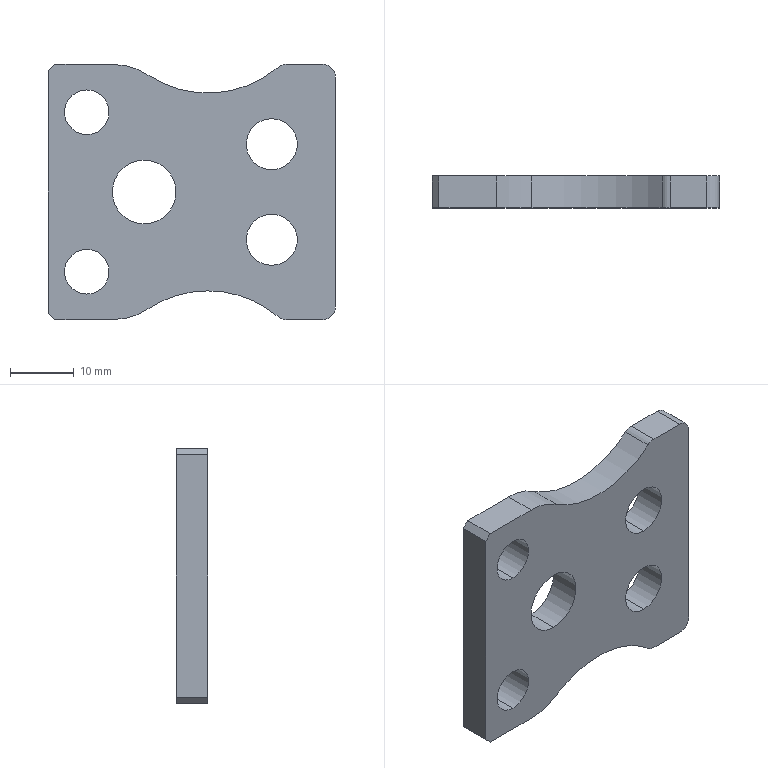Part | SolidWorks | features BaseBody 1 | 1 solid | 29 faces | box 45 x 5 x 40 mm | volume 6983 mm3 | cylinder 19 | plane 10 | commonest cylinder face diameters 4 x4 7 x4 8 x4 34 x3 10 x2 20 x2
STEP:
#1=CARTESIAN_POINT('',(147.5,25.,-3.5));
#2=VERTEX_POINT('',#1);
#3=CARTESIAN_POINT('',(147.5,25.,-11.5));
#4=VERTEX_POINT('',#3);
#5=CARTESIAN_POINT('',(147.5,25.,-7.5));
#6=DIRECTION('',(0.,-1.,0.));
#7=DIRECTION('',(0.,0.,-1.));
#8=AXIS2_PLACEMENT_3D('',#5,#6,#7);
#9=CIRCLE('',#8,4.);
#10=EDGE_CURVE('',#2,#4,#9,.T.);
#11=ORIENTED_EDGE('',*,*,#10,.T.);
#12=CARTESIAN_POINT('',(147.5,30.,-11.5));
#13=VERTEX_POINT('',#12);
#14=CARTESIAN_POINT('',(147.5,25.,-11.5));
#15=DIRECTION('',(0.,1.,0.));
#16=VECTOR('',#15,1000.);
#17=LINE('',#14,#16);
#18=EDGE_CURVE('',#4,#13,#17,.T.);
#19=ORIENTED_EDGE('',*,*,#18,.T.);
#20=CARTESIAN_POINT('',(147.5,30.,-3.5));
#21=VERTEX_POINT('',#20);
#22=CARTESIAN_POINT('',(147.5,30.,-7.5));
#23=DIRECTION('',(0.,-1.,0.));
#24=DIRECTION('',(0.,0.,-1.));
#25=AXIS2_PLACEMENT_3D('',#22,#23,#24);
#26=CIRCLE('',#25,4.);
#27=EDGE_CURVE('',#21,#13,#26,.T.);
#28=ORIENTED_EDGE('',*,*,#27,.F.);
#29=CARTESIAN_POINT('',(147.5,25.,-3.5));
#30=DIRECTION('',(0.,1.,0.));
#31=VECTOR('',#30,1000.);
#32=LINE('',#29,#31);
#33=EDGE_CURVE('',#2,#21,#32,.T.);
#34=ORIENTED_EDGE('',*,*,#33,.F.);
#35=EDGE_LOOP('',(#11,#19,#28,#34));
#36=FACE_OUTER_BOUND('',#35,.T.);
#37=CARTESIAN_POINT('',(147.5,25.,-7.5));
#38=DIRECTION('',(0.,1.,0.));
#39=DIRECTION('',(0.,0.,1.));
#40=AXIS2_PLACEMENT_3D('',#37,#38,#39);
#41=CYLINDRICAL_SURFACE('',#40,4.);
#42=ADVANCED_FACE('',(#36),#41,.F.);
#43=CARTESIAN_POINT('',(147.5,25.,11.5));
#44=VERTEX_POINT('',#43);
#45=CARTESIAN_POINT('',(147.5,25.,3.5));
#46=VERTEX_POINT('',#45);
#47=CARTESIAN_POINT('',(147.5,25.,7.5));
#48=DIRECTION('',(0.,-1.,0.));
#49=DIRECTION('',(0.,0.,-1.));
#50=AXIS2_PLACEMENT_3D('',#47,#48,#49);
#51=CIRCLE('',#50,4.);
#52=EDGE_CURVE('',#44,#46,#51,.T.);
#53=ORIENTED_EDGE('',*,*,#52,.T.);
#54=CARTESIAN_POINT('',(147.5,30.,3.5));
#55=VERTEX_POINT('',#54);
#56=CARTESIAN_POINT('',(147.5,25.,3.5));
#57=DIRECTION('',(0.,1.,0.));
#58=VECTOR('',#57,1000.);
#59=LINE('',#56,#58);
#60=EDGE_CURVE('',#46,#55,#59,.T.);
#61=ORIENTED_EDGE('',*,*,#60,.T.);
#62=CARTESIAN_POINT('',(147.5,30.,11.5));
#63=VERTEX_POINT('',#62);
#64=CARTESIAN_POINT('',(147.5,30.,7.5));
#65=DIRECTION('',(0.,-1.,0.));
#66=DIRECTION('',(0.,0.,-1.));
#67=AXIS2_PLACEMENT_3D('',#64,#65,#66);
#68=CIRCLE('',#67,4.);
#69=EDGE_CURVE('',#63,#55,#68,.T.);
#70=ORIENTED_EDGE('',*,*,#69,.F.);
#71=CARTESIAN_POINT('',(147.5,25.,11.5));
#72=DIRECTION('',(0.,1.,0.));
#73=VECTOR('',#72,1000.);
#74=LINE('',#71,#73);
#75=EDGE_CURVE('',#44,#63,#74,.T.);
#76=ORIENTED_EDGE('',*,*,#75,.F.);
#77=EDGE_LOOP('',(#53,#61,#70,#76));
#78=FACE_OUTER_BOUND('',#77,.T.);
#79=CARTESIAN_POINT('',(147.5,25.,7.5));
#80=DIRECTION('',(0.,1.,0.));
#81=DIRECTION('',(0.,0.,1.));
#82=AXIS2_PLACEMENT_3D('',#79,#80,#81);
#83=CYLINDRICAL_SURFACE('',#82,4.);
#84=ADVANCED_FACE('',(#78),#83,.F.);
#85=CARTESIAN_POINT('',(127.5,25.,5.));
#86=VERTEX_POINT('',#85);
#87=CARTESIAN_POINT('',(127.5,25.,-5.));
#88=VERTEX_POINT('',#87);
#89=CARTESIAN_POINT('',(127.5,25.,0.));
#90=DIRECTION('',(0.,-1.,0.));
#91=DIRECTION('',(0.,0.,-1.));
#92=AXIS2_PLACEMENT_3D('',#89,#90,#91);
#93=CIRCLE('',#92,5.);
#94=EDGE_CURVE('',#86,#88,#93,.T.);
#95=ORIENTED_EDGE('',*,*,#94,.T.);
#96=CARTESIAN_POINT('',(127.5,30.,-5.));
#97=VERTEX_POINT('',#96);
#98=CARTESIAN_POINT('',(127.5,25.,-5.));
#99=DIRECTION('',(0.,1.,0.));
#100=VECTOR('',#99,1000.);
#101=LINE('',#98,#100);
#102=EDGE_CURVE('',#88,#97,#101,.T.);
#103=ORIENTED_EDGE('',*,*,#102,.T.);
#104=CARTESIAN_POINT('',(127.5,30.,5.));
#105=VERTEX_POINT('',#104);
#106=CARTESIAN_POINT('',(127.5,30.,0.));
#107=DIRECTION('',(0.,-1.,0.));
#108=DIRECTION('',(0.,0.,-1.));
#109=AXIS2_PLACEMENT_3D('',#106,#107,#108);
#110=CIRCLE('',#109,5.);
#111=EDGE_CURVE('',#105,#97,#110,.T.);
#112=ORIENTED_EDGE('',*,*,#111,.F.);
#113=CARTESIAN_POINT('',(127.5,25.,5.));
#114=DIRECTION('',(0.,1.,0.));
#115=VECTOR('',#114,1000.);
#116=LINE('',#113,#115);
#117=EDGE_CURVE('',#86,#105,#116,.T.);
#118=ORIENTED_EDGE('',*,*,#117,.F.);
#119=EDGE_LOOP('',(#95,#103,#112,#118));
#120=FACE_OUTER_BOUND('',#119,.T.);
#121=CARTESIAN_POINT('',(127.5,25.,0.));
#122=DIRECTION('',(0.,1.,0.));
#123=DIRECTION('',(0.,0.,1.));
#124=AXIS2_PLACEMENT_3D('',#121,#122,#123);
#125=CYLINDRICAL_SURFACE('',#124,5.);
#126=ADVANCED_FACE('',(#120),#125,.F.);
#127=CARTESIAN_POINT('',(118.5,25.,16.));
#128=VERTEX_POINT('',#127);
#129=CARTESIAN_POINT('',(118.5,25.,9.));
#130=VERTEX_POINT('',#129);
#131=CARTESIAN_POINT('',(118.5,25.,12.5));
#132=DIRECTION('',(0.,-1.,0.));
#133=DIRECTION('',(0.,0.,-1.));
#134=AXIS2_PLACEMENT_3D('',#131,#132,#133);
#135=CIRCLE('',#134,3.5);
#136=EDGE_CURVE('',#128,#130,#135,.T.);
#137=ORIENTED_EDGE('',*,*,#136,.T.);
#138=CARTESIAN_POINT('',(118.5,30.,9.));
#139=VERTEX_POINT('',#138);
#140=CARTESIAN_POINT('',(118.5,25.,9.));
#141=DIRECTION('',(0.,1.,0.));
#142=VECTOR('',#141,1000.);
#143=LINE('',#140,#142);
#144=EDGE_CURVE('',#130,#139,#143,.T.);
#145=ORIENTED_EDGE('',*,*,#144,.T.);
#146=CARTESIAN_POINT('',(118.5,30.,16.));
#147=VERTEX_POINT('',#146);
#148=CARTESIAN_POINT('',(118.5,30.,12.5));
#149=DIRECTION('',(0.,-1.,0.));
#150=DIRECTION('',(0.,0.,-1.));
#151=AXIS2_PLACEMENT_3D('',#148,#149,#150);
#152=CIRCLE('',#151,3.5);
#153=EDGE_CURVE('',#147,#139,#152,.T.);
#154=ORIENTED_EDGE('',*,*,#153,.F.);
#155=CARTESIAN_POINT('',(118.5,25.,16.));
#156=DIRECTION('',(0.,1.,0.));
#157=VECTOR('',#156,1000.);
#158=LINE('',#155,#157);
#159=EDGE_CURVE('',#128,#147,#158,.T.);
#160=ORIENTED_EDGE('',*,*,#159,.F.);
#161=EDGE_LOOP('',(#137,#145,#154,#160));
#162=FACE_OUTER_BOUND('',#161,.T.);
#163=CARTESIAN_POINT('',(118.5,25.,12.5));
#164=DIRECTION('',(0.,1.,0.));
#165=DIRECTION('',(0.,0.,1.));
#166=AXIS2_PLACEMENT_3D('',#163,#164,#165);
#167=CYLINDRICAL_SURFACE('',#166,3.5);
#168=ADVANCED_FACE('',(#162),#167,.F.);
#169=CARTESIAN_POINT('',(118.5,25.,-9.));
#170=VERTEX_POINT('',#169);
#171=CARTESIAN_POINT('',(118.5,25.,-16.));
#172=VERTEX_POINT('',#171);
#173=CARTESIAN_POINT('',(118.5,25.,-12.5));
#174=DIRECTION('',(0.,-1.,0.));
#175=DIRECTION('',(0.,0.,-1.));
#176=AXIS2_PLACEMENT_3D('',#173,#174,#175);
#177=CIRCLE('',#176,3.5);
#178=EDGE_CURVE('',#170,#172,#177,.T.);
#179=ORIENTED_EDGE('',*,*,#178,.T.);
#180=CARTESIAN_POINT('',(118.5,30.,-16.));
#181=VERTEX_POINT('',#180);
#182=CARTESIAN_POINT('',(118.5,25.,-16.));
#183=DIRECTION('',(0.,1.,0.));
#184=VECTOR('',#183,1000.);
#185=LINE('',#182,#184);
#186=EDGE_CURVE('',#172,#181,#185,.T.);
#187=ORIENTED_EDGE('',*,*,#186,.T.);
#188=CARTESIAN_POINT('',(118.5,30.,-9.));
#189=VERTEX_POINT('',#188);
#190=CARTESIAN_POINT('',(118.5,30.,-12.5));
#191=DIRECTION('',(0.,-1.,0.));
#192=DIRECTION('',(0.,0.,-1.));
#193=AXIS2_PLACEMENT_3D('',#190,#191,#192);
#194=CIRCLE('',#193,3.5);
#195=EDGE_CURVE('',#189,#181,#194,.T.);
#196=ORIENTED_EDGE('',*,*,#195,.F.);
#197=CARTESIAN_POINT('',(118.5,25.,-9.));
#198=DIRECTION('',(0.,1.,0.));
#199=VECTOR('',#198,1000.);
#200=LINE('',#197,#199);
#201=EDGE_CURVE('',#170,#189,#200,.T.);
#202=ORIENTED_EDGE('',*,*,#201,.F.);
#203=EDGE_LOOP('',(#179,#187,#196,#202));
#204=FACE_OUTER_BOUND('',#203,.T.);
#205=CARTESIAN_POINT('',(118.5,25.,-12.5));
#206=DIRECTION('',(0.,1.,0.));
#207=DIRECTION('',(0.,0.,1.));
#208=AXIS2_PLACEMENT_3D('',#205,#206,#207);
#209=CYLINDRICAL_SURFACE('',#208,3.5);
#210=ADVANCED_FACE('',(#204),#209,.F.);
#211=CARTESIAN_POINT('',(137.5,25.,-15.5));
#212=VERTEX_POINT('',#211);
#213=CARTESIAN_POINT('',(148.486,25.,-19.526));
#214=VERTEX_POINT('',#213);
#215=CARTESIAN_POINT('',(137.5,25.,-32.5));
#216=DIRECTION('',(0.,1.,0.));
#217=DIRECTION('',(0.,0.,-1.));
#218=AXIS2_PLACEMENT_3D('',#215,#216,#217);
#219=CIRCLE('',#218,17.);
#220=EDGE_CURVE('',#212,#214,#219,.T.);
#221=ORIENTED_EDGE('',*,*,#220,.F.);
#222=CARTESIAN_POINT('',(137.5,30.,-15.5));
#223=VERTEX_POINT('',#222);
#224=CARTESIAN_POINT('',(137.5,25.,-15.5));
#225=DIRECTION('',(0.,1.,0.));
#226=VECTOR('',#225,1000.);
#227=LINE('',#224,#226);
#228=EDGE_CURVE('',#212,#223,#227,.T.);
#229=ORIENTED_EDGE('',*,*,#228,.T.);
#230=CARTESIAN_POINT('',(148.486,30.,-19.526));
#231=VERTEX_POINT('',#230);
#232=CARTESIAN_POINT('',(137.5,30.,-32.5));
#233=DIRECTION('',(0.,1.,0.));
#234=DIRECTION('',(0.,0.,-1.));
#235=AXIS2_PLACEMENT_3D('',#232,#233,#234);
#236=CIRCLE('',#235,17.);
#237=EDGE_CURVE('',#223,#231,#236,.T.);
#238=ORIENTED_EDGE('',*,*,#237,.T.);
#239=CARTESIAN_POINT('',(148.486,25.,-19.526));
#240=DIRECTION('',(0.,1.,0.));
#241=VECTOR('',#240,1000.);
#242=LINE('',#239,#241);
#243=EDGE_CURVE('',#214,#231,#242,.T.);
#244=ORIENTED_EDGE('',*,*,#243,.F.);
#245=EDGE_LOOP('',(#221,#229,#238,#244));
#246=FACE_OUTER_BOUND('',#245,.T.);
#247=CARTESIAN_POINT('',(137.5,25.,-32.5));
#248=DIRECTION('',(0.,1.,0.));
#249=DIRECTION('',(0.,0.,1.));
#250=AXIS2_PLACEMENT_3D('',#247,#248,#249);
#251=CYLINDRICAL_SURFACE('',#250,17.);
#252=ADVANCED_FACE('',(#246),#251,.F.);
#253=CARTESIAN_POINT('',(122.575,30.,-20.));
#254=VERTEX_POINT('',#253);
#255=CARTESIAN_POINT('',(128.103,30.,-18.333));
#256=VERTEX_POINT('',#255);
#257=CARTESIAN_POINT('',(122.575,30.,-10.));
#258=DIRECTION('',(0.,-1.,0.));
#259=DIRECTION('',(0.,0.,-1.));
#260=AXIS2_PLACEMENT_3D('',#257,#258,#259);
#261=CIRCLE('',#260,10.);
#262=EDGE_CURVE('',#254,#256,#261,.T.);
#263=ORIENTED_EDGE('',*,*,#262,.T.);
#264=CARTESIAN_POINT('',(128.103,25.,-18.333));
#265=VERTEX_POINT('',#264);
#266=CARTESIAN_POINT('',(128.103,25.,-18.333));
#267=DIRECTION('',(0.,1.,0.));
#268=VECTOR('',#267,1000.);
#269=LINE('',#266,#268);
#270=EDGE_CURVE('',#265,#256,#269,.T.);
#271=ORIENTED_EDGE('',*,*,#270,.F.);
#272=CARTESIAN_POINT('',(122.575,25.,-20.));
#273=VERTEX_POINT('',#272);
#274=CARTESIAN_POINT('',(122.575,25.,-10.));
#275=DIRECTION('',(0.,-1.,0.));
#276=DIRECTION('',(0.,0.,-1.));
#277=AXIS2_PLACEMENT_3D('',#274,#275,#276);
#278=CIRCLE('',#277,10.);
#279=EDGE_CURVE('',#273,#265,#278,.T.);
#280=ORIENTED_EDGE('',*,*,#279,.F.);
#281=CARTESIAN_POINT('',(122.575,25.,-20.));
#282=DIRECTION('',(0.,1.,0.));
#283=VECTOR('',#282,1000.);
#284=LINE('',#281,#283);
#285=EDGE_CURVE('',#273,#254,#284,.T.);
#286=ORIENTED_EDGE('',*,*,#285,.T.);
#287=EDGE_LOOP('',(#263,#271,#280,#286));
#288=FACE_OUTER_BOUND('',#287,.T.);
#289=CARTESIAN_POINT('',(122.575,25.,-10.));
#290=DIRECTION('',(0.,1.,0.));
#291=DIRECTION('',(0.,0.,1.));
#292=AXIS2_PLACEMENT_3D('',#289,#290,#291);
#293=CYLINDRICAL_SURFACE('',#292,10.);
#294=ADVANCED_FACE('',(#288),#293,.T.);
#295=CARTESIAN_POINT('',(113.5,30.,-20.));
#296=VERTEX_POINT('',#295);
#297=CARTESIAN_POINT('',(113.5,30.,-20.));
#298=DIRECTION('',(1.,0.,0.));
#299=VECTOR('',#298,1000.);
#300=LINE('',#297,#299);
#301=EDGE_CURVE('',#296,#254,#300,.T.);
#302=ORIENTED_EDGE('',*,*,#301,.T.);
#303=ORIENTED_EDGE('',*,*,#285,.F.);
#304=CARTESIAN_POINT('',(113.5,25.,-20.));
#305=VERTEX_POINT('',#304);
#306=CARTESIAN_POINT('',(113.5,25.,-20.));
#307=DIRECTION('',(1.,0.,0.));
#308=VECTOR('',#307,1000.);
#309=LINE('',#306,#308);
#310=EDGE_CURVE('',#305,#273,#309,.T.);
#311=ORIENTED_EDGE('',*,*,#310,.F.);
#312=CARTESIAN_POINT('',(113.5,25.,-20.));
#313=DIRECTION('',(0.,1.,0.));
#314=VECTOR('',#313,1000.);
#315=LINE('',#312,#314);
#316=EDGE_CURVE('',#305,#296,#315,.T.);
#317=ORIENTED_EDGE('',*,*,#316,.T.);
#318=EDGE_LOOP('',(#302,#303,#311,#317));
#319=FACE_OUTER_BOUND('',#318,.T.);
#320=CARTESIAN_POINT('',(113.5,25.,-20.));
#321=DIRECTION('',(0.,0.,1.));
#322=DIRECTION('',(0.,-1.,0.));
#323=AXIS2_PLACEMENT_3D('',#320,#321,#322);
#324=PLANE('',#323);
#325=ADVANCED_FACE('',(#319),#324,.F.);
#326=CARTESIAN_POINT('',(112.5,30.,-19.));
#327=VERTEX_POINT('',#326);
#328=CARTESIAN_POINT('',(112.5,30.,-19.));
#329=DIRECTION('',(0.7071,0.,-0.7071));
#330=VECTOR('',#329,1000.);
#331=LINE('',#328,#330);
#332=EDGE_CURVE('',#327,#296,#331,.T.);
#333=ORIENTED_EDGE('',*,*,#332,.T.);
#334=ORIENTED_EDGE('',*,*,#316,.F.);
#335=CARTESIAN_POINT('',(112.5,25.,-19.));
#336=VERTEX_POINT('',#335);
#337=CARTESIAN_POINT('',(112.5,25.,-19.));
#338=DIRECTION('',(0.7071,0.,-0.7071));
#339=VECTOR('',#338,1000.);
#340=LINE('',#337,#339);
#341=EDGE_CURVE('',#336,#305,#340,.T.);
#342=ORIENTED_EDGE('',*,*,#341,.F.);
#343=CARTESIAN_POINT('',(112.5,25.,-19.));
#344=DIRECTION('',(0.,1.,0.));
#345=VECTOR('',#344,1000.);
#346=LINE('',#343,#345);
#347=EDGE_CURVE('',#336,#327,#346,.T.);
#348=ORIENTED_EDGE('',*,*,#347,.T.);
#349=EDGE_LOOP('',(#333,#334,#342,#348));
#350=FACE_OUTER_BOUND('',#349,.T.);
#351=CARTESIAN_POINT('',(112.5,25.,-19.));
#352=DIRECTION('',(0.7071,0.,0.7071));
#353=DIRECTION('',(0.,-1.,0.));
#354=AXIS2_PLACEMENT_3D('',#351,#352,#353);
#355=PLANE('',#354);
#356=ADVANCED_FACE('',(#350),#355,.F.);
#357=CARTESIAN_POINT('',(112.5,30.,19.));
#358=VERTEX_POINT('',#357);
#359=CARTESIAN_POINT('',(112.5,30.,19.));
#360=DIRECTION('',(0.,0.,-1.));
#361=VECTOR('',#360,1000.);
#362=LINE('',#359,#361);
#363=EDGE_CURVE('',#358,#327,#362,.T.);
#364=ORIENTED_EDGE('',*,*,#363,.T.);
#365=ORIENTED_EDGE('',*,*,#347,.F.);
#366=CARTESIAN_POINT('',(112.5,25.,19.));
#367=VERTEX_POINT('',#366);
#368=CARTESIAN_POINT('',(112.5,25.,19.));
#369=DIRECTION('',(0.,0.,-1.));
#370=VECTOR('',#369,1000.);
#371=LINE('',#368,#370);
#372=EDGE_CURVE('',#367,#336,#371,.T.);
#373=ORIENTED_EDGE('',*,*,#372,.F.);
#374=CARTESIAN_POINT('',(112.5,25.,19.));
#375=DIRECTION('',(0.,1.,0.));
#376=VECTOR('',#375,1000.);
#377=LINE('',#374,#376);
#378=EDGE_CURVE('',#367,#358,#377,.T.);
#379=ORIENTED_EDGE('',*,*,#378,.T.);
#380=EDGE_LOOP('',(#364,#365,#373,#379));
#381=FACE_OUTER_BOUND('',#380,.T.);
#382=CARTESIAN_POINT('',(112.5,25.,19.));
#383=DIRECTION('',(1.,0.,0.));
#384=DIRECTION('',(0.,0.,-1.));
#385=AXIS2_PLACEMENT_3D('',#382,#383,#384);
#386=PLANE('',#385);
#387=ADVANCED_FACE('',(#381),#386,.F.);
#388=CARTESIAN_POINT('',(113.5,30.,20.));
#389=VERTEX_POINT('',#388);
#390=CARTESIAN_POINT('',(113.5,30.,20.));
#391=DIRECTION('',(-0.7071,0.,-0.7071));
#392=VECTOR('',#391,1000.);
#393=LINE('',#390,#392);
#394=EDGE_CURVE('',#389,#358,#393,.T.);
#395=ORIENTED_EDGE('',*,*,#394,.T.);
#396=ORIENTED_EDGE('',*,*,#378,.F.);
#397=CARTESIAN_POINT('',(113.5,25.,20.));
#398=VERTEX_POINT('',#397);
#399=CARTESIAN_POINT('',(113.5,25.,20.));
#400=DIRECTION('',(-0.7071,0.,-0.7071));
#401=VECTOR('',#400,1000.);
#402=LINE('',#399,#401);
#403=EDGE_CURVE('',#398,#367,#402,.T.);
#404=ORIENTED_EDGE('',*,*,#403,.F.);
#405=CARTESIAN_POINT('',(113.5,25.,20.));
#406=DIRECTION('',(0.,1.,0.));
#407=VECTOR('',#406,1000.);
#408=LINE('',#405,#407);
#409=EDGE_CURVE('',#398,#389,#408,.T.);
#410=ORIENTED_EDGE('',*,*,#409,.T.);
#411=EDGE_LOOP('',(#395,#396,#404,#410));
#412=FACE_OUTER_BOUND('',#411,.T.);
#413=CARTESIAN_POINT('',(113.5,25.,20.));
#414=DIRECTION('',(0.7071,0.,-0.7071));
#415=DIRECTION('',(0.,-1.,0.));
#416=AXIS2_PLACEMENT_3D('',#413,#414,#415);
#417=PLANE('',#416);
#418=ADVANCED_FACE('',(#412),#417,.F.);
#419=CARTESIAN_POINT('',(122.575,30.,20.));
#420=VERTEX_POINT('',#419);
#421=CARTESIAN_POINT('',(122.575,30.,20.));
#422=DIRECTION('',(-1.,0.,0.));
#423=VECTOR('',#422,1000.);
#424=LINE('',#421,#423);
#425=EDGE_CURVE('',#420,#389,#424,.T.);
#426=ORIENTED_EDGE('',*,*,#425,.T.);
#427=ORIENTED_EDGE('',*,*,#409,.F.);
#428=CARTESIAN_POINT('',(122.575,25.,20.));
#429=VERTEX_POINT('',#428);
#430=CARTESIAN_POINT('',(122.575,25.,20.));
#431=DIRECTION('',(-1.,0.,0.));
#432=VECTOR('',#431,1000.);
#433=LINE('',#430,#432);
#434=EDGE_CURVE('',#429,#398,#433,.T.);
#435=ORIENTED_EDGE('',*,*,#434,.F.);
#436=CARTESIAN_POINT('',(122.575,25.,20.));
#437=DIRECTION('',(0.,1.,0.));
#438=VECTOR('',#437,1000.);
#439=LINE('',#436,#438);
#440=EDGE_CURVE('',#429,#420,#439,.T.);
#441=ORIENTED_EDGE('',*,*,#440,.T.);
#442=EDGE_LOOP('',(#426,#427,#435,#441));
#443=FACE_OUTER_BOUND('',#442,.T.);
#444=CARTESIAN_POINT('',(122.575,25.,20.));
#445=DIRECTION('',(0.,0.,-1.));
#446=DIRECTION('',(-1.,0.,0.));
#447=AXIS2_PLACEMENT_3D('',#444,#445,#446);
#448=PLANE('',#447);
#449=ADVANCED_FACE('',(#443),#448,.F.);
#450=CARTESIAN_POINT('',(128.103,30.,18.333));
#451=VERTEX_POINT('',#450);
#452=CARTESIAN_POINT('',(122.575,30.,10.));
#453=DIRECTION('',(0.,-1.,0.));
#454=DIRECTION('',(0.,0.,-1.));
#455=AXIS2_PLACEMENT_3D('',#452,#453,#454);
#456=CIRCLE('',#455,10.);
#457=EDGE_CURVE('',#451,#420,#456,.T.);
#458=ORIENTED_EDGE('',*,*,#457,.T.);
#459=ORIENTED_EDGE('',*,*,#440,.F.);
#460=CARTESIAN_POINT('',(128.103,25.,18.333));
#461=VERTEX_POINT('',#460);
#462=CARTESIAN_POINT('',(122.575,25.,10.));
#463=DIRECTION('',(0.,-1.,0.));
#464=DIRECTION('',(0.,0.,-1.));
#465=AXIS2_PLACEMENT_3D('',#462,#463,#464);
#466=CIRCLE('',#465,10.);
#467=EDGE_CURVE('',#461,#429,#466,.T.);
#468=ORIENTED_EDGE('',*,*,#467,.F.);
#469=CARTESIAN_POINT('',(128.103,25.,18.333));
#470=DIRECTION('',(0.,1.,0.));
#471=VECTOR('',#470,1000.);
#472=LINE('',#469,#471);
#473=EDGE_CURVE('',#461,#451,#472,.T.);
#474=ORIENTED_EDGE('',*,*,#473,.T.);
#475=EDGE_LOOP('',(#458,#459,#468,#474));
#476=FACE_OUTER_BOUND('',#475,.T.);
#477=CARTESIAN_POINT('',(122.575,25.,10.));
#478=DIRECTION('',(0.,1.,0.));
#479=DIRECTION('',(0.,0.,1.));
#480=AXIS2_PLACEMENT_3D('',#477,#478,#479);
#481=CYLINDRICAL_SURFACE('',#480,10.);
#482=ADVANCED_FACE('',(#476),#481,.T.);
#483=CARTESIAN_POINT('',(148.486,30.,19.526));
#484=VERTEX_POINT('',#483);
#485=CARTESIAN_POINT('',(137.5,30.,32.5));
#486=DIRECTION('',(0.,1.,0.));
#487=DIRECTION('',(0.,0.,-1.));
#488=AXIS2_PLACEMENT_3D('',#485,#486,#487);
#489=CIRCLE('',#488,17.);
#490=EDGE_CURVE('',#484,#451,#489,.T.);
#491=ORIENTED_EDGE('',*,*,#490,.T.);
#492=ORIENTED_EDGE('',*,*,#473,.F.);
#493=CARTESIAN_POINT('',(148.486,25.,19.526));
#494=VERTEX_POINT('',#493);
#495=CARTESIAN_POINT('',(137.5,25.,32.5));
#496=DIRECTION('',(0.,1.,0.));
#497=DIRECTION('',(0.,0.,-1.));
#498=AXIS2_PLACEMENT_3D('',#495,#496,#497);
#499=CIRCLE('',#498,17.);
#500=EDGE_CURVE('',#494,#461,#499,.T.);
#501=ORIENTED_EDGE('',*,*,#500,.F.);
#502=CARTESIAN_POINT('',(148.486,25.,19.526));
#503=DIRECTION('',(0.,1.,0.));
#504=VECTOR('',#503,1000.);
#505=LINE('',#502,#504);
#506=EDGE_CURVE('',#494,#484,#505,.T.);
#507=ORIENTED_EDGE('',*,*,#506,.T.);
#508=EDGE_LOOP('',(#491,#492,#501,#507));
#509=FACE_OUTER_BOUND('',#508,.T.);
#510=CARTESIAN_POINT('',(137.5,25.,32.5));
#511=DIRECTION('',(0.,1.,0.));
#512=DIRECTION('',(0.,0.,1.));
#513=AXIS2_PLACEMENT_3D('',#510,#511,#512);
#514=CYLINDRICAL_SURFACE('',#513,17.);
#515=ADVANCED_FACE('',(#509),#514,.F.);
#516=CARTESIAN_POINT('',(149.778,30.,20.));
#517=VERTEX_POINT('',#516);
#518=CARTESIAN_POINT('',(149.778,30.,18.));
#519=DIRECTION('',(0.,-1.,0.));
#520=DIRECTION('',(0.,0.,-1.));
#521=AXIS2_PLACEMENT_3D('',#518,#519,#520);
#522=CIRCLE('',#521,2.);
#523=EDGE_CURVE('',#517,#484,#522,.T.);
#524=ORIENTED_EDGE('',*,*,#523,.T.);
#525=ORIENTED_EDGE('',*,*,#506,.F.);
#526=CARTESIAN_POINT('',(149.778,25.,20.));
#527=VERTEX_POINT('',#526);
#528=CARTESIAN_POINT('',(149.778,25.,18.));
#529=DIRECTION('',(0.,-1.,0.));
#530=DIRECTION('',(0.,0.,-1.));
#531=AXIS2_PLACEMENT_3D('',#528,#529,#530);
#532=CIRCLE('',#531,2.);
#533=EDGE_CURVE('',#527,#494,#532,.T.);
#534=ORIENTED_EDGE('',*,*,#533,.F.);
#535=CARTESIAN_POINT('',(149.778,25.,20.));
#536=DIRECTION('',(0.,1.,0.));
#537=VECTOR('',#536,1000.);
#538=LINE('',#535,#537);
#539=EDGE_CURVE('',#527,#517,#538,.T.);
#540=ORIENTED_EDGE('',*,*,#539,.T.);
#541=EDGE_LOOP('',(#524,#525,#534,#540));
#542=FACE_OUTER_BOUND('',#541,.T.);
#543=CARTESIAN_POINT('',(149.778,25.,18.));
#544=DIRECTION('',(0.,1.,0.));
#545=DIRECTION('',(0.,0.,1.));
#546=AXIS2_PLACEMENT_3D('',#543,#544,#545);
#547=CYLINDRICAL_SURFACE('',#546,2.);
#548=ADVANCED_FACE('',(#542),#547,.T.);
#549=CARTESIAN_POINT('',(155.5,30.,20.));
#550=VERTEX_POINT('',#549);
#551=CARTESIAN_POINT('',(155.5,30.,20.));
#552=DIRECTION('',(-1.,0.,0.));
#553=VECTOR('',#552,1000.);
#554=LINE('',#551,#553);
#555=EDGE_CURVE('',#550,#517,#554,.T.);
#556=ORIENTED_EDGE('',*,*,#555,.T.);
#557=ORIENTED_EDGE('',*,*,#539,.F.);
#558=CARTESIAN_POINT('',(155.5,25.,20.));
#559=VERTEX_POINT('',#558);
#560=CARTESIAN_POINT('',(155.5,25.,20.));
#561=DIRECTION('',(-1.,0.,0.));
#562=VECTOR('',#561,1000.);
#563=LINE('',#560,#562);
#564=EDGE_CURVE('',#559,#527,#563,.T.);
#565=ORIENTED_EDGE('',*,*,#564,.F.);
#566=CARTESIAN_POINT('',(155.5,25.,20.));
#567=DIRECTION('',(0.,1.,0.));
#568=VECTOR('',#567,1000.);
#569=LINE('',#566,#568);
#570=EDGE_CURVE('',#559,#550,#569,.T.);
#571=ORIENTED_EDGE('',*,*,#570,.T.);
#572=EDGE_LOOP('',(#556,#557,#565,#571));
#573=FACE_OUTER_BOUND('',#572,.T.);
#574=CARTESIAN_POINT('',(155.5,25.,20.));
#575=DIRECTION('',(0.,0.,-1.));
#576=DIRECTION('',(-1.,0.,0.));
#577=AXIS2_PLACEMENT_3D('',#574,#575,#576);
#578=PLANE('',#577);
#579=ADVANCED_FACE('',(#573),#578,.F.);
#580=CARTESIAN_POINT('',(157.5,30.,18.));
#581=VERTEX_POINT('',#580);
#582=CARTESIAN_POINT('',(155.5,30.,18.));
#583=DIRECTION('',(0.,-1.,0.));
#584=DIRECTION('',(0.,0.,-1.));
#585=AXIS2_PLACEMENT_3D('',#582,#583,#584);
#586=CIRCLE('',#585,2.);
#587=EDGE_CURVE('',#581,#550,#586,.T.);
#588=ORIENTED_EDGE('',*,*,#587,.T.);
#589=ORIENTED_EDGE('',*,*,#570,.F.);
#590=CARTESIAN_POINT('',(157.5,25.,18.));
#591=VERTEX_POINT('',#590);
#592=CARTESIAN_POINT('',(155.5,25.,18.));
#593=DIRECTION('',(0.,-1.,0.));
#594=DIRECTION('',(0.,0.,-1.));
#595=AXIS2_PLACEMENT_3D('',#592,#593,#594);
#596=CIRCLE('',#595,2.);
#597=EDGE_CURVE('',#591,#559,#596,.T.);
#598=ORIENTED_EDGE('',*,*,#597,.F.);
#599=CARTESIAN_POINT('',(157.5,25.,18.));
#600=DIRECTION('',(0.,1.,0.));
#601=VECTOR('',#600,1000.);
#602=LINE('',#599,#601);
#603=EDGE_CURVE('',#591,#581,#602,.T.);
#604=ORIENTED_EDGE('',*,*,#603,.T.);
#605=EDGE_LOOP('',(#588,#589,#598,#604));
#606=FACE_OUTER_BOUND('',#605,.T.);
#607=CARTESIAN_POINT('',(155.5,25.,18.));
#608=DIRECTION('',(0.,1.,0.));
#609=DIRECTION('',(0.,0.,1.));
#610=AXIS2_PLACEMENT_3D('',#607,#608,#609);
#611=CYLINDRICAL_SURFACE('',#610,2.);
#612=ADVANCED_FACE('',(#606),#611,.T.);
#613=CARTESIAN_POINT('',(157.5,30.,-18.));
#614=VERTEX_POINT('',#613);
#615=CARTESIAN_POINT('',(157.5,30.,-18.));
#616=DIRECTION('',(0.,0.,1.));
#617=VECTOR('',#616,1000.);
#618=LINE('',#615,#617);
#619=EDGE_CURVE('',#614,#581,#618,.T.);
#620=ORIENTED_EDGE('',*,*,#619,.T.);
#621=ORIENTED_EDGE('',*,*,#603,.F.);
#622=CARTESIAN_POINT('',(157.5,25.,-18.));
#623=VERTEX_POINT('',#622);
#624=CARTESIAN_POINT('',(157.5,25.,-18.));
#625=DIRECTION('',(0.,0.,1.));
#626=VECTOR('',#625,1000.);
#627=LINE('',#624,#626);
#628=EDGE_CURVE('',#623,#591,#627,.T.);
#629=ORIENTED_EDGE('',*,*,#628,.F.);
#630=CARTESIAN_POINT('',(157.5,25.,-18.));
#631=DIRECTION('',(0.,1.,0.));
#632=VECTOR('',#631,1000.);
#633=LINE('',#630,#632);
#634=EDGE_CURVE('',#623,#614,#633,.T.);
#635=ORIENTED_EDGE('',*,*,#634,.T.);
#636=EDGE_LOOP('',(#620,#621,#629,#635));
#637=FACE_OUTER_BOUND('',#636,.T.);
#638=CARTESIAN_POINT('',(157.5,25.,-18.));
#639=DIRECTION('',(-1.,0.,0.));
#640=DIRECTION('',(0.,1.,0.));
#641=AXIS2_PLACEMENT_3D('',#638,#639,#640);
#642=PLANE('',#641);
#643=ADVANCED_FACE('',(#637),#642,.F.);
#644=CARTESIAN_POINT('',(155.5,30.,-20.));
#645=VERTEX_POINT('',#644);
#646=CARTESIAN_POINT('',(155.5,30.,-18.));
#647=DIRECTION('',(0.,-1.,0.));
#648=DIRECTION('',(0.,0.,-1.));
#649=AXIS2_PLACEMENT_3D('',#646,#647,#648);
#650=CIRCLE('',#649,2.);
#651=EDGE_CURVE('',#645,#614,#650,.T.);
#652=ORIENTED_EDGE('',*,*,#651,.T.);
#653=ORIENTED_EDGE('',*,*,#634,.F.);
#654=CARTESIAN_POINT('',(155.5,25.,-20.));
#655=VERTEX_POINT('',#654);
#656=CARTESIAN_POINT('',(155.5,25.,-18.));
#657=DIRECTION('',(0.,-1.,0.));
#658=DIRECTION('',(0.,0.,-1.));
#659=AXIS2_PLACEMENT_3D('',#656,#657,#658);
#660=CIRCLE('',#659,2.);
#661=EDGE_CURVE('',#655,#623,#660,.T.);
#662=ORIENTED_EDGE('',*,*,#661,.F.);
#663=CARTESIAN_POINT('',(155.5,25.,-20.));
#664=DIRECTION('',(0.,1.,0.));
#665=VECTOR('',#664,1000.);
#666=LINE('',#663,#665);
#667=EDGE_CURVE('',#655,#645,#666,.T.);
#668=ORIENTED_EDGE('',*,*,#667,.T.);
#669=EDGE_LOOP('',(#652,#653,#662,#668));
#670=FACE_OUTER_BOUND('',#669,.T.);
#671=CARTESIAN_POINT('',(155.5,25.,-18.));
#672=DIRECTION('',(0.,1.,0.));
#673=DIRECTION('',(0.,0.,1.));
#674=AXIS2_PLACEMENT_3D('',#671,#672,#673);
#675=CYLINDRICAL_SURFACE('',#674,2.);
#676=ADVANCED_FACE('',(#670),#675,.T.);
#677=CARTESIAN_POINT('',(149.778,30.,-20.));
#678=VERTEX_POINT('',#677);
#679=CARTESIAN_POINT('',(149.778,30.,-20.));
#680=DIRECTION('',(1.,0.,0.));
#681=VECTOR('',#680,1000.);
#682=LINE('',#679,#681);
#683=EDGE_CURVE('',#678,#645,#682,.T.);
#684=ORIENTED_EDGE('',*,*,#683,.T.);
#685=ORIENTED_EDGE('',*,*,#667,.F.);
#686=CARTESIAN_POINT('',(149.778,25.,-20.));
#687=VERTEX_POINT('',#686);
#688=CARTESIAN_POINT('',(149.778,25.,-20.));
#689=DIRECTION('',(1.,0.,0.));
#690=VECTOR('',#689,1000.);
#691=LINE('',#688,#690);
#692=EDGE_CURVE('',#687,#655,#691,.T.);
#693=ORIENTED_EDGE('',*,*,#692,.F.);
#694=CARTESIAN_POINT('',(149.778,25.,-20.));
#695=DIRECTION('',(0.,1.,0.));
#696=VECTOR('',#695,1000.);
#697=LINE('',#694,#696);
#698=EDGE_CURVE('',#687,#678,#697,.T.);
#699=ORIENTED_EDGE('',*,*,#698,.T.);
#700=EDGE_LOOP('',(#684,#685,#693,#699));
#701=FACE_OUTER_BOUND('',#700,.T.);
#702=CARTESIAN_POINT('',(149.778,25.,-20.));
#703=DIRECTION('',(0.,0.,1.));
#704=DIRECTION('',(0.,-1.,0.));
#705=AXIS2_PLACEMENT_3D('',#702,#703,#704);
#706=PLANE('',#705);
#707=ADVANCED_FACE('',(#701),#706,.F.);
#708=CARTESIAN_POINT('',(149.778,30.,-18.));
#709=DIRECTION('',(0.,-1.,0.));
#710=DIRECTION('',(0.,0.,-1.));
#711=AXIS2_PLACEMENT_3D('',#708,#709,#710);
#712=CIRCLE('',#711,2.);
#713=EDGE_CURVE('',#231,#678,#712,.T.);
#714=ORIENTED_EDGE('',*,*,#713,.T.);
#715=ORIENTED_EDGE('',*,*,#698,.F.);
#716=CARTESIAN_POINT('',(149.778,25.,-18.));
#717=DIRECTION('',(0.,-1.,0.));
#718=DIRECTION('',(0.,0.,-1.));
#719=AXIS2_PLACEMENT_3D('',#716,#717,#718);
#720=CIRCLE('',#719,2.);
#721=EDGE_CURVE('',#214,#687,#720,.T.);
#722=ORIENTED_EDGE('',*,*,#721,.F.);
#723=ORIENTED_EDGE('',*,*,#243,.T.);
#724=EDGE_LOOP('',(#714,#715,#722,#723));
#725=FACE_OUTER_BOUND('',#724,.T.);
#726=CARTESIAN_POINT('',(149.778,25.,-18.));
#727=DIRECTION('',(0.,1.,0.));
#728=DIRECTION('',(0.,0.,1.));
#729=AXIS2_PLACEMENT_3D('',#726,#727,#728);
#730=CYLINDRICAL_SURFACE('',#729,2.);
#731=ADVANCED_FACE('',(#725),#730,.T.);
#732=ORIENTED_EDGE('',*,*,#27,.T.);
#733=CARTESIAN_POINT('',(147.5,30.,-7.5));
#734=DIRECTION('',(0.,-1.,0.));
#735=DIRECTION('',(0.,0.,-1.));
#736=AXIS2_PLACEMENT_3D('',#733,#734,#735);
#737=CIRCLE('',#736,4.);
#738=EDGE_CURVE('',#13,#21,#737,.T.);
#739=ORIENTED_EDGE('',*,*,#738,.T.);
#740=EDGE_LOOP('',(#732,#739));
#741=FACE_BOUND('',#740,.T.);
#742=ORIENTED_EDGE('',*,*,#69,.T.);
#743=CARTESIAN_POINT('',(147.5,30.,7.5));
#744=DIRECTION('',(0.,-1.,0.));
#745=DIRECTION('',(0.,0.,-1.));
#746=AXIS2_PLACEMENT_3D('',#743,#744,#745);
#747=CIRCLE('',#746,4.);
#748=EDGE_CURVE('',#55,#63,#747,.T.);
#749=ORIENTED_EDGE('',*,*,#748,.T.);
#750=EDGE_LOOP('',(#742,#749));
#751=FACE_BOUND('',#750,.T.);
#752=ORIENTED_EDGE('',*,*,#111,.T.);
#753=CARTESIAN_POINT('',(127.5,30.,0.));
#754=DIRECTION('',(0.,-1.,0.));
#755=DIRECTION('',(0.,0.,-1.));
#756=AXIS2_PLACEMENT_3D('',#753,#754,#755);
#757=CIRCLE('',#756,5.);
#758=EDGE_CURVE('',#97,#105,#757,.T.);
#759=ORIENTED_EDGE('',*,*,#758,.T.);
#760=EDGE_LOOP('',(#752,#759));
#761=FACE_BOUND('',#760,.T.);
#762=ORIENTED_EDGE('',*,*,#153,.T.);
#763=CARTESIAN_POINT('',(118.5,30.,12.5));
#764=DIRECTION('',(0.,-1.,0.));
#765=DIRECTION('',(0.,0.,-1.));
#766=AXIS2_PLACEMENT_3D('',#763,#764,#765);
#767=CIRCLE('',#766,3.5);
#768=EDGE_CURVE('',#139,#147,#767,.T.);
#769=ORIENTED_EDGE('',*,*,#768,.T.);
#770=EDGE_LOOP('',(#762,#769));
#771=FACE_BOUND('',#770,.T.);
#772=ORIENTED_EDGE('',*,*,#195,.T.);
#773=CARTESIAN_POINT('',(118.5,30.,-12.5));
#774=DIRECTION('',(0.,-1.,0.));
#775=DIRECTION('',(0.,0.,-1.));
#776=AXIS2_PLACEMENT_3D('',#773,#774,#775);
#777=CIRCLE('',#776,3.5);
#778=EDGE_CURVE('',#181,#189,#777,.T.);
#779=ORIENTED_EDGE('',*,*,#778,.T.);
#780=EDGE_LOOP('',(#772,#779));
#781=FACE_BOUND('',#780,.T.);
#782=ORIENTED_EDGE('',*,*,#713,.F.);
#783=ORIENTED_EDGE('',*,*,#237,.F.);
#784=CARTESIAN_POINT('',(137.5,30.,-32.5));
#785=DIRECTION('',(0.,1.,0.));
#786=DIRECTION('',(0.,0.,-1.));
#787=AXIS2_PLACEMENT_3D('',#784,#785,#786);
#788=CIRCLE('',#787,17.);
#789=EDGE_CURVE('',#256,#223,#788,.T.);
#790=ORIENTED_EDGE('',*,*,#789,.F.);
#791=ORIENTED_EDGE('',*,*,#262,.F.);
#792=ORIENTED_EDGE('',*,*,#301,.F.);
#793=ORIENTED_EDGE('',*,*,#332,.F.);
#794=ORIENTED_EDGE('',*,*,#363,.F.);
#795=ORIENTED_EDGE('',*,*,#394,.F.);
#796=ORIENTED_EDGE('',*,*,#425,.F.);
#797=ORIENTED_EDGE('',*,*,#457,.F.);
#798=ORIENTED_EDGE('',*,*,#490,.F.);
#799=ORIENTED_EDGE('',*,*,#523,.F.);
#800=ORIENTED_EDGE('',*,*,#555,.F.);
#801=ORIENTED_EDGE('',*,*,#587,.F.);
#802=ORIENTED_EDGE('',*,*,#619,.F.);
#803=ORIENTED_EDGE('',*,*,#651,.F.);
#804=ORIENTED_EDGE('',*,*,#683,.F.);
#805=EDGE_LOOP('',(#782,#783,#790,#791,#792,#793,#794,#795,#796,#797,#798,#799,#800,#801,#802,#803,#804));
#806=FACE_OUTER_BOUND('',#805,.T.);
#807=CARTESIAN_POINT('',(149.778,30.,-18.));
#808=DIRECTION('',(0.,-1.,0.));
#809=DIRECTION('',(0.,0.,-1.));
#810=AXIS2_PLACEMENT_3D('',#807,#808,#809);
#811=PLANE('',#810);
#812=ADVANCED_FACE('',(#741,#751,#761,#771,#781,#806),#811,.F.);
#813=ORIENTED_EDGE('',*,*,#10,.F.);
#814=CARTESIAN_POINT('',(147.5,25.,-7.5));
#815=DIRECTION('',(0.,-1.,0.));
#816=DIRECTION('',(0.,0.,-1.));
#817=AXIS2_PLACEMENT_3D('',#814,#815,#816);
#818=CIRCLE('',#817,4.);
#819=EDGE_CURVE('',#4,#2,#818,.T.);
#820=ORIENTED_EDGE('',*,*,#819,.F.);
#821=EDGE_LOOP('',(#813,#820));
#822=FACE_BOUND('',#821,.T.);
#823=ORIENTED_EDGE('',*,*,#94,.F.);
#824=CARTESIAN_POINT('',(127.5,25.,0.));
#825=DIRECTION('',(0.,-1.,0.));
#826=DIRECTION('',(0.,0.,-1.));
#827=AXIS2_PLACEMENT_3D('',#824,#825,#826);
#828=CIRCLE('',#827,5.);
#829=EDGE_CURVE('',#88,#86,#828,.T.);
#830=ORIENTED_EDGE('',*,*,#829,.F.);
#831=EDGE_LOOP('',(#823,#830));
#832=FACE_BOUND('',#831,.T.);
#833=ORIENTED_EDGE('',*,*,#178,.F.);
#834=CARTESIAN_POINT('',(118.5,25.,-12.5));
#835=DIRECTION('',(0.,-1.,0.));
#836=DIRECTION('',(0.,0.,-1.));
#837=AXIS2_PLACEMENT_3D('',#834,#835,#836);
#838=CIRCLE('',#837,3.5);
#839=EDGE_CURVE('',#172,#170,#838,.T.);
#840=ORIENTED_EDGE('',*,*,#839,.F.);
#841=EDGE_LOOP('',(#833,#840));
#842=FACE_BOUND('',#841,.T.);
#843=ORIENTED_EDGE('',*,*,#136,.F.);
#844=CARTESIAN_POINT('',(118.5,25.,12.5));
#845=DIRECTION('',(0.,-1.,0.));
#846=DIRECTION('',(0.,0.,-1.));
#847=AXIS2_PLACEMENT_3D('',#844,#845,#846);
#848=CIRCLE('',#847,3.5);
#849=EDGE_CURVE('',#130,#128,#848,.T.);
#850=ORIENTED_EDGE('',*,*,#849,.F.);
#851=EDGE_LOOP('',(#843,#850));
#852=FACE_BOUND('',#851,.T.);
#853=ORIENTED_EDGE('',*,*,#52,.F.);
#854=CARTESIAN_POINT('',(147.5,25.,7.5));
#855=DIRECTION('',(0.,-1.,0.));
#856=DIRECTION('',(0.,0.,-1.));
#857=AXIS2_PLACEMENT_3D('',#854,#855,#856);
#858=CIRCLE('',#857,4.);
#859=EDGE_CURVE('',#46,#44,#858,.T.);
#860=ORIENTED_EDGE('',*,*,#859,.F.);
#861=EDGE_LOOP('',(#853,#860));
#862=FACE_BOUND('',#861,.T.);
#863=ORIENTED_EDGE('',*,*,#721,.T.);
#864=ORIENTED_EDGE('',*,*,#692,.T.);
#865=ORIENTED_EDGE('',*,*,#661,.T.);
#866=ORIENTED_EDGE('',*,*,#628,.T.);
#867=ORIENTED_EDGE('',*,*,#597,.T.);
#868=ORIENTED_EDGE('',*,*,#564,.T.);
#869=ORIENTED_EDGE('',*,*,#533,.T.);
#870=ORIENTED_EDGE('',*,*,#500,.T.);
#871=ORIENTED_EDGE('',*,*,#467,.T.);
#872=ORIENTED_EDGE('',*,*,#434,.T.);
#873=ORIENTED_EDGE('',*,*,#403,.T.);
#874=ORIENTED_EDGE('',*,*,#372,.T.);
#875=ORIENTED_EDGE('',*,*,#341,.T.);
#876=ORIENTED_EDGE('',*,*,#310,.T.);
#877=ORIENTED_EDGE('',*,*,#279,.T.);
#878=CARTESIAN_POINT('',(137.5,25.,-32.5));
#879=DIRECTION('',(0.,1.,0.));
#880=DIRECTION('',(0.,0.,-1.));
#881=AXIS2_PLACEMENT_3D('',#878,#879,#880);
#882=CIRCLE('',#881,17.);
#883=EDGE_CURVE('',#265,#212,#882,.T.);
#884=ORIENTED_EDGE('',*,*,#883,.T.);
#885=ORIENTED_EDGE('',*,*,#220,.T.);
#886=EDGE_LOOP('',(#863,#864,#865,#866,#867,#868,#869,#870,#871,#872,#873,#874,#875,#876,#877,#884,#885));
#887=FACE_OUTER_BOUND('',#886,.T.);
#888=CARTESIAN_POINT('',(149.778,25.,-18.));
#889=DIRECTION('',(0.,-1.,0.));
#890=DIRECTION('',(0.,0.,-1.));
#891=AXIS2_PLACEMENT_3D('',#888,#889,#890);
#892=PLANE('',#891);
#893=ADVANCED_FACE('',(#822,#832,#842,#852,#862,#887),#892,.T.);
#894=ORIENTED_EDGE('',*,*,#228,.F.);
#895=ORIENTED_EDGE('',*,*,#883,.F.);
#896=ORIENTED_EDGE('',*,*,#270,.T.);
#897=ORIENTED_EDGE('',*,*,#789,.T.);
#898=EDGE_LOOP('',(#894,#895,#896,#897));
#899=FACE_OUTER_BOUND('',#898,.T.);
#900=CARTESIAN_POINT('',(137.5,25.,-32.5));
#901=DIRECTION('',(0.,1.,0.));
#902=DIRECTION('',(0.,0.,1.));
#903=AXIS2_PLACEMENT_3D('',#900,#901,#902);
#904=CYLINDRICAL_SURFACE('',#903,17.);
#905=ADVANCED_FACE('',(#899),#904,.F.);
#906=ORIENTED_EDGE('',*,*,#186,.F.);
#907=ORIENTED_EDGE('',*,*,#839,.T.);
#908=ORIENTED_EDGE('',*,*,#201,.T.);
#909=ORIENTED_EDGE('',*,*,#778,.F.);
#910=EDGE_LOOP('',(#906,#907,#908,#909));
#911=FACE_OUTER_BOUND('',#910,.T.);
#912=CARTESIAN_POINT('',(118.5,25.,-12.5));
#913=DIRECTION('',(0.,1.,0.));
#914=DIRECTION('',(0.,0.,1.));
#915=AXIS2_PLACEMENT_3D('',#912,#913,#914);
#916=CYLINDRICAL_SURFACE('',#915,3.5);
#917=ADVANCED_FACE('',(#911),#916,.F.);
#918=ORIENTED_EDGE('',*,*,#144,.F.);
#919=ORIENTED_EDGE('',*,*,#849,.T.);
#920=ORIENTED_EDGE('',*,*,#159,.T.);
#921=ORIENTED_EDGE('',*,*,#768,.F.);
#922=EDGE_LOOP('',(#918,#919,#920,#921));
#923=FACE_OUTER_BOUND('',#922,.T.);
#924=CARTESIAN_POINT('',(118.5,25.,12.5));
#925=DIRECTION('',(0.,1.,0.));
#926=DIRECTION('',(0.,0.,1.));
#927=AXIS2_PLACEMENT_3D('',#924,#925,#926);
#928=CYLINDRICAL_SURFACE('',#927,3.5);
#929=ADVANCED_FACE('',(#923),#928,.F.);
#930=ORIENTED_EDGE('',*,*,#102,.F.);
#931=ORIENTED_EDGE('',*,*,#829,.T.);
#932=ORIENTED_EDGE('',*,*,#117,.T.);
#933=ORIENTED_EDGE('',*,*,#758,.F.);
#934=EDGE_LOOP('',(#930,#931,#932,#933));
#935=FACE_OUTER_BOUND('',#934,.T.);
#936=CARTESIAN_POINT('',(127.5,25.,0.));
#937=DIRECTION('',(0.,1.,0.));
#938=DIRECTION('',(0.,0.,1.));
#939=AXIS2_PLACEMENT_3D('',#936,#937,#938);
#940=CYLINDRICAL_SURFACE('',#939,5.);
#941=ADVANCED_FACE('',(#935),#940,.F.);
#942=ORIENTED_EDGE('',*,*,#60,.F.);
#943=ORIENTED_EDGE('',*,*,#859,.T.);
#944=ORIENTED_EDGE('',*,*,#75,.T.);
#945=ORIENTED_EDGE('',*,*,#748,.F.);
#946=EDGE_LOOP('',(#942,#943,#944,#945));
#947=FACE_OUTER_BOUND('',#946,.T.);
#948=CARTESIAN_POINT('',(147.5,25.,7.5));
#949=DIRECTION('',(0.,1.,0.));
#950=DIRECTION('',(0.,0.,1.));
#951=AXIS2_PLACEMENT_3D('',#948,#949,#950);
#952=CYLINDRICAL_SURFACE('',#951,4.);
#953=ADVANCED_FACE('',(#947),#952,.F.);
#954=ORIENTED_EDGE('',*,*,#18,.F.);
#955=ORIENTED_EDGE('',*,*,#819,.T.);
#956=ORIENTED_EDGE('',*,*,#33,.T.);
#957=ORIENTED_EDGE('',*,*,#738,.F.);
#958=EDGE_LOOP('',(#954,#955,#956,#957));
#959=FACE_OUTER_BOUND('',#958,.T.);
#960=CARTESIAN_POINT('',(147.5,25.,-7.5));
#961=DIRECTION('',(0.,1.,0.));
#962=DIRECTION('',(0.,0.,1.));
#963=AXIS2_PLACEMENT_3D('',#960,#961,#962);
#964=CYLINDRICAL_SURFACE('',#963,4.);
#965=ADVANCED_FACE('',(#959),#964,.F.);
#966=CLOSED_SHELL('',(#42,#84,#126,#168,#210,#252,#294,#325,#356,#387,#418,#449,#482,#515,#548,#579,#612,#643,#676,#707,#731,#812,#893,#905,#917,#929,#941,#953,#965));
#967=MANIFOLD_SOLID_BREP('',#966);
#968=CARTESIAN_POINT('',(0.,0.,0.));
#969=DIRECTION('',(0.,0.,1.));
#970=DIRECTION('',(1.,0.,0.));
#971=AXIS2_PLACEMENT_3D('',#968,#969,#970);
#972=(LENGTH_UNIT()NAMED_UNIT(*)SI_UNIT(.MILLI.,.METRE.));
#973=UNCERTAINTY_MEASURE_WITH_UNIT(LENGTH_MEASURE(0.00001),#972,'','');
#974=(NAMED_UNIT(*)PLANE_ANGLE_UNIT()SI_UNIT($,.RADIAN.));
#975=(NAMED_UNIT(*)SI_UNIT($,.STERADIAN.)SOLID_ANGLE_UNIT());
#976=(GEOMETRIC_REPRESENTATION_CONTEXT(3)GLOBAL_UNCERTAINTY_ASSIGNED_CONTEXT((#973))GLOBAL_UNIT_ASSIGNED_CONTEXT((#972,#974,#975))REPRESENTATION_CONTEXT('',''));
#977=ADVANCED_BREP_SHAPE_REPRESENTATION('',(#967,#971),#976);